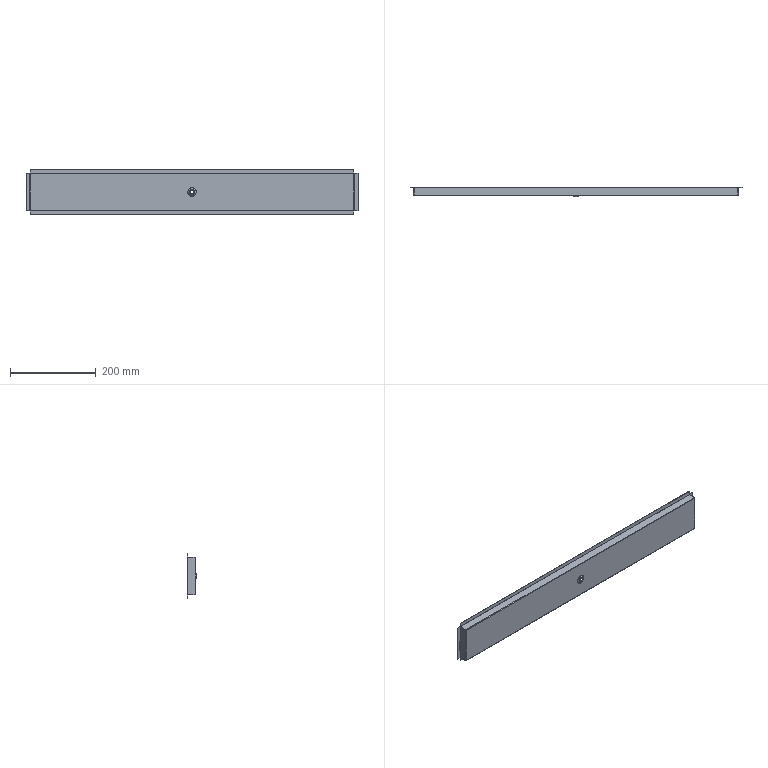Part | STEP file | HESS-408-70-15W-W-26-lower door drip tray | 1 solid | 70 faces | box 776 x 23 x 106 mm | volume 113085 mm3 | plane 40 | cylinder 18 | spline 8 | cone 4 | commonest cylinder face diameters 0.2 x8 2.2 x8 8 x2